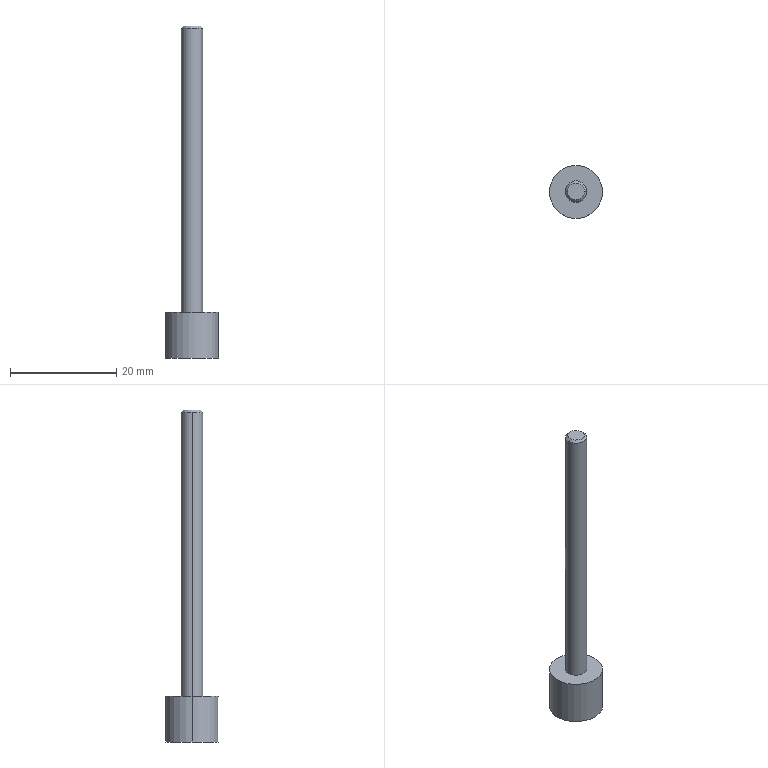Part | SolidWorks | features BaseBody 1 | 1 solid | 9 faces | box 10 x 10 x 62.6 mm | volume 1353 mm3 | cylinder 4 | plane 3 | cone 2 | commonest cylinder face diameters 4 x2 10 x2
STEP:
#1=CARTESIAN_POINT('',(-2.,0.,34.17));
#2=VERTEX_POINT('',#1);
#3=CARTESIAN_POINT('',(2.,0.,34.17));
#4=VERTEX_POINT('',#3);
#5=CARTESIAN_POINT('',(0.,0.,34.17));
#6=DIRECTION('',(0.,0.,-1.));
#7=DIRECTION('',(-1.,0.,0.));
#8=AXIS2_PLACEMENT_3D('',#5,#6,#7);
#9=CIRCLE('',#8,2.);
#10=EDGE_CURVE('',#2,#4,#9,.T.);
#11=ORIENTED_EDGE('',*,*,#10,.T.);
#12=CARTESIAN_POINT('',(2.,0.,-19.4));
#13=VERTEX_POINT('',#12);
#14=CARTESIAN_POINT('',(2.,0.,7.385));
#15=DIRECTION('',(0.,0.,-1.));
#16=VECTOR('',#15,1000.);
#17=LINE('',#14,#16);
#18=EDGE_CURVE('',#4,#13,#17,.T.);
#19=ORIENTED_EDGE('',*,*,#18,.T.);
#20=CARTESIAN_POINT('',(-2.,0.,-19.4));
#21=VERTEX_POINT('',#20);
#22=CARTESIAN_POINT('',(0.,0.,-19.4));
#23=DIRECTION('',(0.,0.,1.));
#24=DIRECTION('',(-1.,0.,0.));
#25=AXIS2_PLACEMENT_3D('',#22,#23,#24);
#26=CIRCLE('',#25,2.);
#27=EDGE_CURVE('',#13,#21,#26,.T.);
#28=ORIENTED_EDGE('',*,*,#27,.T.);
#29=CARTESIAN_POINT('',(-2.,0.,7.385));
#30=DIRECTION('',(0.,0.,-1.));
#31=VECTOR('',#30,1000.);
#32=LINE('',#29,#31);
#33=EDGE_CURVE('',#2,#21,#32,.T.);
#34=ORIENTED_EDGE('',*,*,#33,.F.);
#35=EDGE_LOOP('',(#11,#19,#28,#34));
#36=FACE_OUTER_BOUND('',#35,.T.);
#37=CARTESIAN_POINT('',(0.,0.,7.385));
#38=DIRECTION('',(0.,0.,-1.));
#39=DIRECTION('',(-1.,0.,0.));
#40=AXIS2_PLACEMENT_3D('',#37,#38,#39);
#41=CYLINDRICAL_SURFACE('',#40,2.);
#42=ADVANCED_FACE('',(#36),#41,.T.);
#43=CARTESIAN_POINT('',(-1.571,0.,34.6));
#44=VERTEX_POINT('',#43);
#45=CARTESIAN_POINT('',(1.571,0.,34.6));
#46=VERTEX_POINT('',#45);
#47=CARTESIAN_POINT('',(0.,0.,34.6));
#48=DIRECTION('',(0.,0.,-1.));
#49=DIRECTION('',(-1.,0.,0.));
#50=AXIS2_PLACEMENT_3D('',#47,#48,#49);
#51=CIRCLE('',#50,1.571);
#52=EDGE_CURVE('',#44,#46,#51,.T.);
#53=ORIENTED_EDGE('',*,*,#52,.T.);
#54=CARTESIAN_POINT('',(2.,0.,34.171));
#55=DIRECTION('',(0.7071,0.,-0.7071));
#56=VECTOR('',#55,1000.);
#57=LINE('',#54,#56);
#58=EDGE_CURVE('',#46,#4,#57,.T.);
#59=ORIENTED_EDGE('',*,*,#58,.T.);
#60=ORIENTED_EDGE('',*,*,#10,.F.);
#61=CARTESIAN_POINT('',(-2.,0.,34.171));
#62=DIRECTION('',(-0.7071,0.,-0.7071));
#63=VECTOR('',#62,1000.);
#64=LINE('',#61,#63);
#65=EDGE_CURVE('',#44,#2,#64,.T.);
#66=ORIENTED_EDGE('',*,*,#65,.F.);
#67=EDGE_LOOP('',(#53,#59,#60,#66));
#68=FACE_OUTER_BOUND('',#67,.T.);
#69=CARTESIAN_POINT('',(0.,0.,34.171));
#70=DIRECTION('',(0.,0.,-1.));
#71=DIRECTION('',(-1.,0.,0.));
#72=AXIS2_PLACEMENT_3D('',#69,#70,#71);
#73=CONICAL_SURFACE('',#72,2.,0.7854);
#74=ADVANCED_FACE('',(#68),#73,.T.);
#75=CARTESIAN_POINT('',(5.,0.,-19.4));
#76=VERTEX_POINT('',#75);
#77=CARTESIAN_POINT('',(-5.,0.,-19.4));
#78=VERTEX_POINT('',#77);
#79=CARTESIAN_POINT('',(0.,0.,-19.4));
#80=DIRECTION('',(0.,0.,1.));
#81=DIRECTION('',(-1.,0.,0.));
#82=AXIS2_PLACEMENT_3D('',#79,#80,#81);
#83=CIRCLE('',#82,5.);
#84=EDGE_CURVE('',#76,#78,#83,.T.);
#85=ORIENTED_EDGE('',*,*,#84,.F.);
#86=CARTESIAN_POINT('',(5.,0.,-28.));
#87=VERTEX_POINT('',#86);
#88=CARTESIAN_POINT('',(5.,0.,-23.7));
#89=DIRECTION('',(0.,0.,-1.));
#90=VECTOR('',#89,1000.);
#91=LINE('',#88,#90);
#92=EDGE_CURVE('',#76,#87,#91,.T.);
#93=ORIENTED_EDGE('',*,*,#92,.T.);
#94=CARTESIAN_POINT('',(-5.,0.,-28.));
#95=VERTEX_POINT('',#94);
#96=CARTESIAN_POINT('',(0.,0.,-28.));
#97=DIRECTION('',(0.,0.,1.));
#98=DIRECTION('',(-1.,0.,0.));
#99=AXIS2_PLACEMENT_3D('',#96,#97,#98);
#100=CIRCLE('',#99,5.);
#101=EDGE_CURVE('',#87,#95,#100,.T.);
#102=ORIENTED_EDGE('',*,*,#101,.T.);
#103=CARTESIAN_POINT('',(-5.,0.,-23.7));
#104=DIRECTION('',(0.,0.,-1.));
#105=VECTOR('',#104,1000.);
#106=LINE('',#103,#105);
#107=EDGE_CURVE('',#78,#95,#106,.T.);
#108=ORIENTED_EDGE('',*,*,#107,.F.);
#109=EDGE_LOOP('',(#85,#93,#102,#108));
#110=FACE_OUTER_BOUND('',#109,.T.);
#111=CARTESIAN_POINT('',(0.,0.,-23.7));
#112=DIRECTION('',(0.,0.,-1.));
#113=DIRECTION('',(-1.,0.,0.));
#114=AXIS2_PLACEMENT_3D('',#111,#112,#113);
#115=CYLINDRICAL_SURFACE('',#114,5.);
#116=ADVANCED_FACE('',(#110),#115,.T.);
#117=ORIENTED_EDGE('',*,*,#18,.F.);
#118=CARTESIAN_POINT('',(0.,0.,34.17));
#119=DIRECTION('',(0.,0.,-1.));
#120=DIRECTION('',(-1.,0.,0.));
#121=AXIS2_PLACEMENT_3D('',#118,#119,#120);
#122=CIRCLE('',#121,2.);
#123=EDGE_CURVE('',#4,#2,#122,.T.);
#124=ORIENTED_EDGE('',*,*,#123,.T.);
#125=ORIENTED_EDGE('',*,*,#33,.T.);
#126=CARTESIAN_POINT('',(0.,0.,-19.4));
#127=DIRECTION('',(0.,0.,1.));
#128=DIRECTION('',(-1.,0.,0.));
#129=AXIS2_PLACEMENT_3D('',#126,#127,#128);
#130=CIRCLE('',#129,2.);
#131=EDGE_CURVE('',#21,#13,#130,.T.);
#132=ORIENTED_EDGE('',*,*,#131,.T.);
#133=EDGE_LOOP('',(#117,#124,#125,#132));
#134=FACE_OUTER_BOUND('',#133,.T.);
#135=CARTESIAN_POINT('',(0.,0.,7.385));
#136=DIRECTION('',(0.,0.,-1.));
#137=DIRECTION('',(-1.,0.,0.));
#138=AXIS2_PLACEMENT_3D('',#135,#136,#137);
#139=CYLINDRICAL_SURFACE('',#138,2.);
#140=ADVANCED_FACE('',(#134),#139,.T.);
#141=ORIENTED_EDGE('',*,*,#58,.F.);
#142=CARTESIAN_POINT('',(0.,0.,34.6));
#143=DIRECTION('',(0.,0.,-1.));
#144=DIRECTION('',(-1.,0.,0.));
#145=AXIS2_PLACEMENT_3D('',#142,#143,#144);
#146=CIRCLE('',#145,1.571);
#147=EDGE_CURVE('',#46,#44,#146,.T.);
#148=ORIENTED_EDGE('',*,*,#147,.T.);
#149=ORIENTED_EDGE('',*,*,#65,.T.);
#150=ORIENTED_EDGE('',*,*,#123,.F.);
#151=EDGE_LOOP('',(#141,#148,#149,#150));
#152=FACE_OUTER_BOUND('',#151,.T.);
#153=CARTESIAN_POINT('',(0.,0.,34.171));
#154=DIRECTION('',(0.,0.,-1.));
#155=DIRECTION('',(-1.,0.,0.));
#156=AXIS2_PLACEMENT_3D('',#153,#154,#155);
#157=CONICAL_SURFACE('',#156,2.,0.7854);
#158=ADVANCED_FACE('',(#152),#157,.T.);
#159=CARTESIAN_POINT('',(0.,0.,-19.4));
#160=DIRECTION('',(0.,0.,1.));
#161=DIRECTION('',(-1.,0.,0.));
#162=AXIS2_PLACEMENT_3D('',#159,#160,#161);
#163=CIRCLE('',#162,5.);
#164=EDGE_CURVE('',#78,#76,#163,.T.);
#165=ORIENTED_EDGE('',*,*,#164,.T.);
#166=ORIENTED_EDGE('',*,*,#84,.T.);
#167=EDGE_LOOP('',(#165,#166));
#168=FACE_OUTER_BOUND('',#167,.T.);
#169=ORIENTED_EDGE('',*,*,#131,.F.);
#170=ORIENTED_EDGE('',*,*,#27,.F.);
#171=EDGE_LOOP('',(#169,#170));
#172=FACE_BOUND('',#171,.T.);
#173=CARTESIAN_POINT('',(0.,3.5,-19.4));
#174=DIRECTION('',(0.,0.,1.));
#175=DIRECTION('',(1.,0.,0.));
#176=AXIS2_PLACEMENT_3D('',#173,#174,#175);
#177=PLANE('',#176);
#178=ADVANCED_FACE('',(#168,#172),#177,.T.);
#179=ORIENTED_EDGE('',*,*,#52,.F.);
#180=ORIENTED_EDGE('',*,*,#147,.F.);
#181=EDGE_LOOP('',(#179,#180));
#182=FACE_OUTER_BOUND('',#181,.T.);
#183=CARTESIAN_POINT('',(0.,0.7853,34.6));
#184=DIRECTION('',(0.,0.,1.));
#185=DIRECTION('',(1.,0.,0.));
#186=AXIS2_PLACEMENT_3D('',#183,#184,#185);
#187=PLANE('',#186);
#188=ADVANCED_FACE('',(#182),#187,.T.);
#189=ORIENTED_EDGE('',*,*,#92,.F.);
#190=ORIENTED_EDGE('',*,*,#164,.F.);
#191=ORIENTED_EDGE('',*,*,#107,.T.);
#192=CARTESIAN_POINT('',(0.,0.,-28.));
#193=DIRECTION('',(0.,0.,1.));
#194=DIRECTION('',(-1.,0.,0.));
#195=AXIS2_PLACEMENT_3D('',#192,#193,#194);
#196=CIRCLE('',#195,5.);
#197=EDGE_CURVE('',#95,#87,#196,.T.);
#198=ORIENTED_EDGE('',*,*,#197,.T.);
#199=EDGE_LOOP('',(#189,#190,#191,#198));
#200=FACE_OUTER_BOUND('',#199,.T.);
#201=CARTESIAN_POINT('',(0.,0.,-23.7));
#202=DIRECTION('',(0.,0.,-1.));
#203=DIRECTION('',(-1.,0.,0.));
#204=AXIS2_PLACEMENT_3D('',#201,#202,#203);
#205=CYLINDRICAL_SURFACE('',#204,5.);
#206=ADVANCED_FACE('',(#200),#205,.T.);
#207=ORIENTED_EDGE('',*,*,#197,.F.);
#208=ORIENTED_EDGE('',*,*,#101,.F.);
#209=EDGE_LOOP('',(#207,#208));
#210=FACE_OUTER_BOUND('',#209,.T.);
#211=CARTESIAN_POINT('',(0.,2.5,-28.));
#212=DIRECTION('',(0.,0.,-1.));
#213=DIRECTION('',(-1.,0.,0.));
#214=AXIS2_PLACEMENT_3D('',#211,#212,#213);
#215=PLANE('',#214);
#216=ADVANCED_FACE('',(#210),#215,.T.);
#217=CLOSED_SHELL('',(#42,#74,#116,#140,#158,#178,#188,#206,#216));
#218=MANIFOLD_SOLID_BREP('',#217);
#219=CARTESIAN_POINT('',(0.,0.,0.));
#220=DIRECTION('',(0.,0.,1.));
#221=DIRECTION('',(1.,0.,0.));
#222=AXIS2_PLACEMENT_3D('',#219,#220,#221);
#223=(LENGTH_UNIT()NAMED_UNIT(*)SI_UNIT(.MILLI.,.METRE.));
#224=UNCERTAINTY_MEASURE_WITH_UNIT(LENGTH_MEASURE(0.00001),#223,'','');
#225=(NAMED_UNIT(*)PLANE_ANGLE_UNIT()SI_UNIT($,.RADIAN.));
#226=(NAMED_UNIT(*)SI_UNIT($,.STERADIAN.)SOLID_ANGLE_UNIT());
#227=(GEOMETRIC_REPRESENTATION_CONTEXT(3)GLOBAL_UNCERTAINTY_ASSIGNED_CONTEXT((#224))GLOBAL_UNIT_ASSIGNED_CONTEXT((#223,#225,#226))REPRESENTATION_CONTEXT('',''));
#228=ADVANCED_BREP_SHAPE_REPRESENTATION('',(#218,#222),#227);